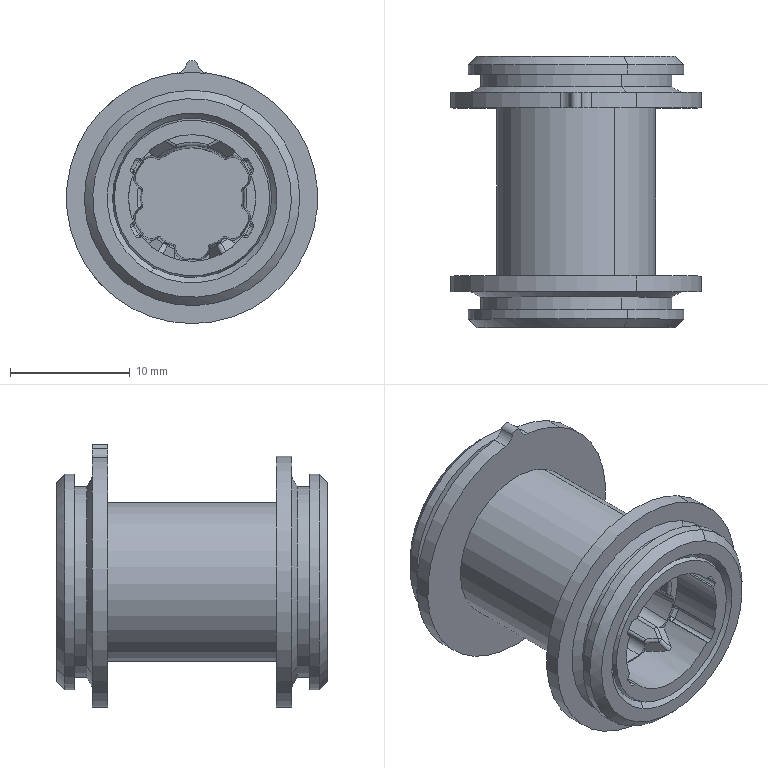Part | NX | features BREP 1 | 1 solid | 380 faces | box 21 x 22.65 x 22 mm | volume 2492 mm3 | cylinder 181 | plane 72 | spline 62 | cone 32 | torus 17 | sphere 16 | commonest cylinder face diameters 0.6 x54 1 x21 1.6 x15 10.6 x12 0.647 x10 10.166 x10